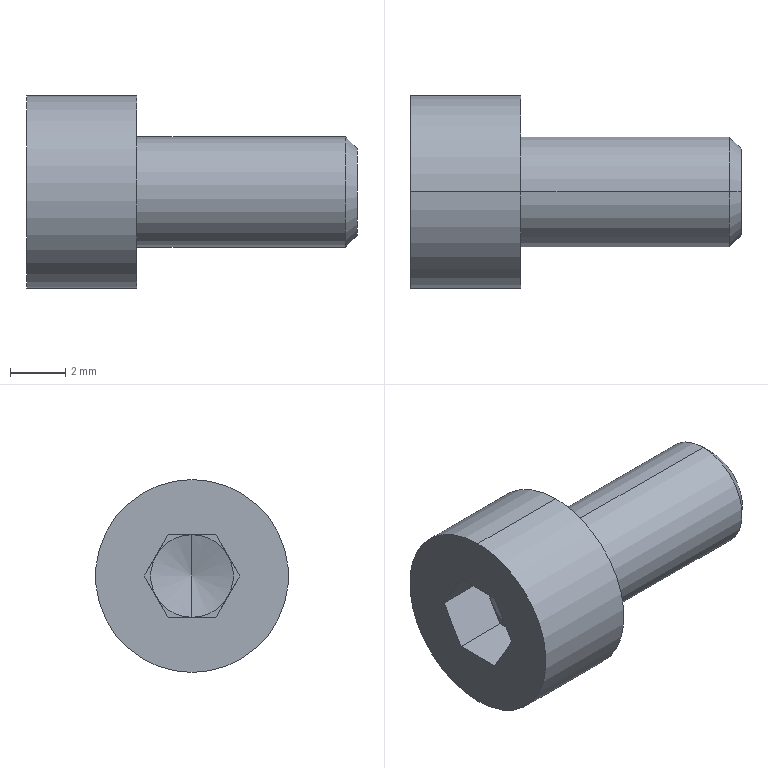Part | STEP file | 0232_303_CBM4-8 | 1 solid | 23 faces | box 12 x 7 x 7 mm | volume 236.857 mm3 | plane 15 | cylinder 4 | cone 4 | commonest cylinder face diameters 4 x2 7 x2
STEP:
#1=CARTESIAN_POINT('',(0.,0.,0.));
#2=DIRECTION('',(0.,0.,1.));
#3=DIRECTION('',(1.,0.,0.));
#4=AXIS2_PLACEMENT_3D('',#1,#2,#3);
#5=CARTESIAN_POINT('',(0.,0.,-2.));
#6=VERTEX_POINT('',#5);
#7=CARTESIAN_POINT('',(0.,0.,2.));
#8=VERTEX_POINT('',#7);
#9=CARTESIAN_POINT('',(0.,0.,0.));
#10=DIRECTION('',(1.,0.,0.));
#11=DIRECTION('',(0.,0.,-1.));
#12=AXIS2_PLACEMENT_3D('',#9,#10,#11);
#13=CIRCLE('',#12,2.);
#14=CARTESIAN_POINT('',(3.785,0.,0.));
#15=DIRECTION('',(1.,0.,0.));
#16=DIRECTION('',(0.,0.,-1.));
#17=AXIS2_PLACEMENT_3D('',#14,#15,#16);
#18=CYLINDRICAL_SURFACE('',#17,2.);
#19=CARTESIAN_POINT('',(0.,-3.785));
#20=DIRECTION('',(1.,0.));
#21=VECTOR('',#20,1.);
#22=LINE('',#19,#21);
#23=(GEOMETRIC_REPRESENTATION_CONTEXT(2)PARAMETRIC_REPRESENTATION_CONTEXT()REPRESENTATION_CONTEXT('',''));
#24=DEFINITIONAL_REPRESENTATION('',(#22),#23);
#25=PCURVE('',#18,#24);
#26=CARTESIAN_POINT('',(0.,2.75,0.));
#27=DIRECTION('',(1.,0.,0.));
#28=DIRECTION('',(0.,0.,-1.));
#29=AXIS2_PLACEMENT_3D('',#26,#27,#28);
#30=PLANE('',#29);
#31=CARTESIAN_POINT('',(0.,-2.75));
#32=DIRECTION('',(1.,0.));
#33=AXIS2_PLACEMENT_2D('',#31,#32);
#34=CIRCLE('',#33,2.);
#35=(GEOMETRIC_REPRESENTATION_CONTEXT(2)PARAMETRIC_REPRESENTATION_CONTEXT()REPRESENTATION_CONTEXT('',''));
#36=DEFINITIONAL_REPRESENTATION('',(#34),#35);
#37=PCURVE('',#30,#36);
#38=SURFACE_CURVE('',#13,(#25,#37),.PCURVE_S1.);
#39=EDGE_CURVE('',#6,#8,#38,.T.);
#40=ORIENTED_EDGE('',*,*,#39,.T.);
#41=CARTESIAN_POINT('',(7.571,0.,2.));
#42=VERTEX_POINT('',#41);
#43=CARTESIAN_POINT('',(3.785,0.,2.));
#44=DIRECTION('',(1.,0.,0.));
#45=VECTOR('',#44,1.);
#46=LINE('',#43,#45);
#47=CARTESIAN_POINT('',(3.142,0.));
#48=DIRECTION('',(0.,1.));
#49=VECTOR('',#48,1.);
#50=LINE('',#47,#49);
#51=(GEOMETRIC_REPRESENTATION_CONTEXT(2)PARAMETRIC_REPRESENTATION_CONTEXT()REPRESENTATION_CONTEXT('',''));
#52=DEFINITIONAL_REPRESENTATION('',(#50),#51);
#53=PCURVE('',#18,#52);
#54=CARTESIAN_POINT('',(3.785,0.,0.));
#55=DIRECTION('',(1.,0.,0.));
#56=DIRECTION('',(0.,0.,-1.));
#57=AXIS2_PLACEMENT_3D('',#54,#55,#56);
#58=CYLINDRICAL_SURFACE('',#57,2.);
#59=CARTESIAN_POINT('',(3.142,0.));
#60=DIRECTION('',(0.,1.));
#61=VECTOR('',#60,1.);
#62=LINE('',#59,#61);
#63=(GEOMETRIC_REPRESENTATION_CONTEXT(2)PARAMETRIC_REPRESENTATION_CONTEXT()REPRESENTATION_CONTEXT('',''));
#64=DEFINITIONAL_REPRESENTATION('',(#62),#63);
#65=PCURVE('',#58,#64);
#66=SURFACE_CURVE('',#46,(#53,#65),.PCURVE_S1.);
#67=EDGE_CURVE('',#8,#42,#66,.T.);
#68=ORIENTED_EDGE('',*,*,#67,.T.);
#69=CARTESIAN_POINT('',(7.571,0.,-2.));
#70=VERTEX_POINT('',#69);
#71=CARTESIAN_POINT('',(7.571,0.,0.));
#72=DIRECTION('',(-1.,0.,0.));
#73=DIRECTION('',(0.,0.,-1.));
#74=AXIS2_PLACEMENT_3D('',#71,#72,#73);
#75=CIRCLE('',#74,2.);
#76=CARTESIAN_POINT('',(6.283,3.785));
#77=DIRECTION('',(-1.,0.));
#78=VECTOR('',#77,1.);
#79=LINE('',#76,#78);
#80=(GEOMETRIC_REPRESENTATION_CONTEXT(2)PARAMETRIC_REPRESENTATION_CONTEXT()REPRESENTATION_CONTEXT('',''));
#81=DEFINITIONAL_REPRESENTATION('',(#79),#80);
#82=PCURVE('',#18,#81);
#83=CARTESIAN_POINT('',(7.571,0.,0.));
#84=DIRECTION('',(-1.,0.,0.));
#85=DIRECTION('',(0.,0.,1.));
#86=AXIS2_PLACEMENT_3D('',#83,#84,#85);
#87=CONICAL_SURFACE('',#86,2.,0.7854);
#88=CARTESIAN_POINT('',(-3.142,0.));
#89=DIRECTION('',(1.,0.));
#90=VECTOR('',#89,1.);
#91=LINE('',#88,#90);
#92=(GEOMETRIC_REPRESENTATION_CONTEXT(2)PARAMETRIC_REPRESENTATION_CONTEXT()REPRESENTATION_CONTEXT('',''));
#93=DEFINITIONAL_REPRESENTATION('',(#91),#92);
#94=PCURVE('',#87,#93);
#95=SURFACE_CURVE('',#75,(#82,#94),.PCURVE_S1.);
#96=EDGE_CURVE('',#42,#70,#95,.T.);
#97=ORIENTED_EDGE('',*,*,#96,.T.);
#98=CARTESIAN_POINT('',(3.785,0.,-2.));
#99=DIRECTION('',(1.,0.,0.));
#100=VECTOR('',#99,1.);
#101=LINE('',#98,#100);
#102=CARTESIAN_POINT('',(0.,0.));
#103=DIRECTION('',(0.,1.));
#104=VECTOR('',#103,1.);
#105=LINE('',#102,#104);
#106=(GEOMETRIC_REPRESENTATION_CONTEXT(2)PARAMETRIC_REPRESENTATION_CONTEXT()REPRESENTATION_CONTEXT('',''));
#107=DEFINITIONAL_REPRESENTATION('',(#105),#106);
#108=PCURVE('',#18,#107);
#109=CARTESIAN_POINT('',(6.283,0.));
#110=DIRECTION('',(0.,1.));
#111=VECTOR('',#110,1.);
#112=LINE('',#109,#111);
#113=(GEOMETRIC_REPRESENTATION_CONTEXT(2)PARAMETRIC_REPRESENTATION_CONTEXT()REPRESENTATION_CONTEXT('',''));
#114=DEFINITIONAL_REPRESENTATION('',(#112),#113);
#115=PCURVE('',#58,#114);
#116=SURFACE_CURVE('',#101,(#108,#115),.PCURVE_S1.);
#117=EDGE_CURVE('',#6,#70,#116,.T.);
#118=ORIENTED_EDGE('',*,*,#117,.F.);
#119=EDGE_LOOP('',(#40,#68,#97,#118));
#120=FACE_BOUND('',#119,.T.);
#121=ADVANCED_FACE('',(#120),#18,.T.);
#122=CARTESIAN_POINT('',(8.,0.,1.571));
#123=VERTEX_POINT('',#122);
#124=CARTESIAN_POINT('',(8.,0.,-1.571));
#125=VERTEX_POINT('',#124);
#126=CARTESIAN_POINT('',(8.,0.,0.));
#127=DIRECTION('',(-1.,0.,0.));
#128=DIRECTION('',(0.,0.,1.));
#129=AXIS2_PLACEMENT_3D('',#126,#127,#128);
#130=CIRCLE('',#129,1.571);
#131=CARTESIAN_POINT('',(0.,-0.4295));
#132=DIRECTION('',(1.,0.));
#133=VECTOR('',#132,1.);
#134=LINE('',#131,#133);
#135=(GEOMETRIC_REPRESENTATION_CONTEXT(2)PARAMETRIC_REPRESENTATION_CONTEXT()REPRESENTATION_CONTEXT('',''));
#136=DEFINITIONAL_REPRESENTATION('',(#134),#135);
#137=PCURVE('',#87,#136);
#138=CARTESIAN_POINT('',(8.,0.7853,0.));
#139=DIRECTION('',(1.,0.,0.));
#140=DIRECTION('',(0.,0.,-1.));
#141=AXIS2_PLACEMENT_3D('',#138,#139,#140);
#142=PLANE('',#141);
#143=CARTESIAN_POINT('',(-1.571,-0.7853));
#144=CARTESIAN_POINT('',(-1.571,1.935));
#145=CARTESIAN_POINT('',(0.7853,0.5748));
#146=CARTESIAN_POINT('',(3.141,-0.7853));
#147=CARTESIAN_POINT('',(0.7853,-2.145));
#148=CARTESIAN_POINT('',(-1.571,-3.505));
#149=CARTESIAN_POINT('',(-1.571,-0.7853));
#150=(BOUNDED_CURVE()B_SPLINE_CURVE(2,(#143,#144,#145,#146,#147,#148,#149),.UNSPECIFIED.,.T.,.F.)B_SPLINE_CURVE_WITH_KNOTS((1,2,2,2,2,1),(-2.094,0.,2.094,4.189,6.283,8.378),.UNSPECIFIED.)CURVE()GEOMETRIC_REPRESENTATION_ITEM()RATIONAL_B_SPLINE_CURVE((1.,0.5,1.,0.5,1.,0.5,1.))REPRESENTATION_ITEM(''));
#151=(GEOMETRIC_REPRESENTATION_CONTEXT(2)PARAMETRIC_REPRESENTATION_CONTEXT()REPRESENTATION_CONTEXT('',''));
#152=DEFINITIONAL_REPRESENTATION('',(#150),#151);
#153=PCURVE('',#142,#152);
#154=SURFACE_CURVE('',#130,(#137,#153),.PCURVE_S1.);
#155=EDGE_CURVE('',#123,#125,#154,.T.);
#156=ORIENTED_EDGE('',*,*,#155,.T.);
#157=CARTESIAN_POINT('',(7.571,0.,-2.));
#158=DIRECTION('',(-0.7071,0.,-0.7071));
#159=VECTOR('',#158,1.);
#160=LINE('',#157,#159);
#161=CARTESIAN_POINT('',(3.142,0.));
#162=DIRECTION('',(0.,1.));
#163=VECTOR('',#162,1.);
#164=LINE('',#161,#163);
#165=(GEOMETRIC_REPRESENTATION_CONTEXT(2)PARAMETRIC_REPRESENTATION_CONTEXT()REPRESENTATION_CONTEXT('',''));
#166=DEFINITIONAL_REPRESENTATION('',(#164),#165);
#167=PCURVE('',#87,#166);
#168=CARTESIAN_POINT('',(7.571,0.,0.));
#169=DIRECTION('',(-1.,0.,0.));
#170=DIRECTION('',(0.,0.,1.));
#171=AXIS2_PLACEMENT_3D('',#168,#169,#170);
#172=CONICAL_SURFACE('',#171,2.,0.7854);
#173=CARTESIAN_POINT('',(3.142,0.));
#174=DIRECTION('',(0.,1.));
#175=VECTOR('',#174,1.);
#176=LINE('',#173,#175);
#177=(GEOMETRIC_REPRESENTATION_CONTEXT(2)PARAMETRIC_REPRESENTATION_CONTEXT()REPRESENTATION_CONTEXT('',''));
#178=DEFINITIONAL_REPRESENTATION('',(#176),#177);
#179=PCURVE('',#172,#178);
#180=SURFACE_CURVE('',#160,(#167,#179),.PCURVE_S1.);
#181=EDGE_CURVE('',#125,#70,#180,.T.);
#182=ORIENTED_EDGE('',*,*,#181,.T.);
#183=ORIENTED_EDGE('',*,*,#96,.F.);
#184=CARTESIAN_POINT('',(7.571,0.,2.));
#185=DIRECTION('',(-0.7071,0.,0.7071));
#186=VECTOR('',#185,1.);
#187=LINE('',#184,#186);
#188=CARTESIAN_POINT('',(0.,0.));
#189=DIRECTION('',(0.,1.));
#190=VECTOR('',#189,1.);
#191=LINE('',#188,#190);
#192=(GEOMETRIC_REPRESENTATION_CONTEXT(2)PARAMETRIC_REPRESENTATION_CONTEXT()REPRESENTATION_CONTEXT('',''));
#193=DEFINITIONAL_REPRESENTATION('',(#191),#192);
#194=PCURVE('',#87,#193);
#195=CARTESIAN_POINT('',(6.283,0.));
#196=DIRECTION('',(0.,1.));
#197=VECTOR('',#196,1.);
#198=LINE('',#195,#197);
#199=(GEOMETRIC_REPRESENTATION_CONTEXT(2)PARAMETRIC_REPRESENTATION_CONTEXT()REPRESENTATION_CONTEXT('',''));
#200=DEFINITIONAL_REPRESENTATION('',(#198),#199);
#201=PCURVE('',#172,#200);
#202=SURFACE_CURVE('',#187,(#194,#201),.PCURVE_S1.);
#203=EDGE_CURVE('',#123,#42,#202,.T.);
#204=ORIENTED_EDGE('',*,*,#203,.F.);
#205=EDGE_LOOP('',(#156,#182,#183,#204));
#206=FACE_BOUND('',#205,.T.);
#207=ADVANCED_FACE('',(#206),#87,.T.);
#208=CARTESIAN_POINT('',(-4.,0.,-3.5));
#209=VERTEX_POINT('',#208);
#210=CARTESIAN_POINT('',(-4.,0.,3.5));
#211=VERTEX_POINT('',#210);
#212=CARTESIAN_POINT('',(-4.,0.,0.));
#213=DIRECTION('',(1.,0.,0.));
#214=DIRECTION('',(0.,0.,-1.));
#215=AXIS2_PLACEMENT_3D('',#212,#213,#214);
#216=CIRCLE('',#215,3.5);
#217=CARTESIAN_POINT('',(-2.,0.,0.));
#218=DIRECTION('',(1.,0.,0.));
#219=DIRECTION('',(0.,0.,-1.));
#220=AXIS2_PLACEMENT_3D('',#217,#218,#219);
#221=CYLINDRICAL_SURFACE('',#220,3.5);
#222=CARTESIAN_POINT('',(0.,-2.));
#223=DIRECTION('',(1.,0.));
#224=VECTOR('',#223,1.);
#225=LINE('',#222,#224);
#226=(GEOMETRIC_REPRESENTATION_CONTEXT(2)PARAMETRIC_REPRESENTATION_CONTEXT()REPRESENTATION_CONTEXT('',''));
#227=DEFINITIONAL_REPRESENTATION('',(#225),#226);
#228=PCURVE('',#221,#227);
#229=CARTESIAN_POINT('',(-4.,1.75,0.));
#230=DIRECTION('',(-1.,0.,0.));
#231=DIRECTION('',(0.,0.,1.));
#232=AXIS2_PLACEMENT_3D('',#229,#230,#231);
#233=PLANE('',#232);
#234=CARTESIAN_POINT('',(-3.5,-1.75));
#235=CARTESIAN_POINT('',(-3.5,4.312));
#236=CARTESIAN_POINT('',(1.75,1.281));
#237=CARTESIAN_POINT('',(7.,-1.75));
#238=CARTESIAN_POINT('',(1.75,-4.781));
#239=CARTESIAN_POINT('',(-3.5,-7.812));
#240=CARTESIAN_POINT('',(-3.5,-1.75));
#241=(BOUNDED_CURVE()B_SPLINE_CURVE(2,(#234,#235,#236,#237,#238,#239,#240),.UNSPECIFIED.,.T.,.F.)B_SPLINE_CURVE_WITH_KNOTS((1,2,2,2,2,1),(-2.094,0.,2.094,4.189,6.283,8.378),.UNSPECIFIED.)CURVE()GEOMETRIC_REPRESENTATION_ITEM()RATIONAL_B_SPLINE_CURVE((1.,0.5,1.,0.5,1.,0.5,1.))REPRESENTATION_ITEM(''));
#242=(GEOMETRIC_REPRESENTATION_CONTEXT(2)PARAMETRIC_REPRESENTATION_CONTEXT()REPRESENTATION_CONTEXT('',''));
#243=DEFINITIONAL_REPRESENTATION('',(#241),#242);
#244=PCURVE('',#233,#243);
#245=SURFACE_CURVE('',#216,(#228,#244),.PCURVE_S1.);
#246=EDGE_CURVE('',#209,#211,#245,.T.);
#247=ORIENTED_EDGE('',*,*,#246,.T.);
#248=CARTESIAN_POINT('',(0.,0.,3.5));
#249=VERTEX_POINT('',#248);
#250=CARTESIAN_POINT('',(-2.,0.,3.5));
#251=DIRECTION('',(1.,0.,0.));
#252=VECTOR('',#251,1.);
#253=LINE('',#250,#252);
#254=CARTESIAN_POINT('',(3.142,0.));
#255=DIRECTION('',(0.,1.));
#256=VECTOR('',#255,1.);
#257=LINE('',#254,#256);
#258=(GEOMETRIC_REPRESENTATION_CONTEXT(2)PARAMETRIC_REPRESENTATION_CONTEXT()REPRESENTATION_CONTEXT('',''));
#259=DEFINITIONAL_REPRESENTATION('',(#257),#258);
#260=PCURVE('',#221,#259);
#261=CARTESIAN_POINT('',(-2.,0.,0.));
#262=DIRECTION('',(1.,0.,0.));
#263=DIRECTION('',(0.,0.,-1.));
#264=AXIS2_PLACEMENT_3D('',#261,#262,#263);
#265=CYLINDRICAL_SURFACE('',#264,3.5);
#266=CARTESIAN_POINT('',(3.142,0.));
#267=DIRECTION('',(0.,1.));
#268=VECTOR('',#267,1.);
#269=LINE('',#266,#268);
#270=(GEOMETRIC_REPRESENTATION_CONTEXT(2)PARAMETRIC_REPRESENTATION_CONTEXT()REPRESENTATION_CONTEXT('',''));
#271=DEFINITIONAL_REPRESENTATION('',(#269),#270);
#272=PCURVE('',#265,#271);
#273=SURFACE_CURVE('',#253,(#260,#272),.PCURVE_S1.);
#274=EDGE_CURVE('',#211,#249,#273,.T.);
#275=ORIENTED_EDGE('',*,*,#274,.T.);
#276=CARTESIAN_POINT('',(0.,0.,-3.5));
#277=VERTEX_POINT('',#276);
#278=CARTESIAN_POINT('',(0.,0.,0.));
#279=DIRECTION('',(1.,0.,0.));
#280=DIRECTION('',(0.,0.,-1.));
#281=AXIS2_PLACEMENT_3D('',#278,#279,#280);
#282=CIRCLE('',#281,3.5);
#283=CARTESIAN_POINT('',(0.,2.));
#284=DIRECTION('',(1.,0.));
#285=VECTOR('',#284,1.);
#286=LINE('',#283,#285);
#287=(GEOMETRIC_REPRESENTATION_CONTEXT(2)PARAMETRIC_REPRESENTATION_CONTEXT()REPRESENTATION_CONTEXT('',''));
#288=DEFINITIONAL_REPRESENTATION('',(#286),#287);
#289=PCURVE('',#221,#288);
#290=CARTESIAN_POINT('',(0.,-2.75));
#291=DIRECTION('',(1.,0.));
#292=AXIS2_PLACEMENT_2D('',#290,#291);
#293=CIRCLE('',#292,3.5);
#294=(GEOMETRIC_REPRESENTATION_CONTEXT(2)PARAMETRIC_REPRESENTATION_CONTEXT()REPRESENTATION_CONTEXT('',''));
#295=DEFINITIONAL_REPRESENTATION('',(#293),#294);
#296=PCURVE('',#30,#295);
#297=SURFACE_CURVE('',#282,(#289,#296),.PCURVE_S1.);
#298=EDGE_CURVE('',#277,#249,#297,.T.);
#299=ORIENTED_EDGE('',*,*,#298,.F.);
#300=CARTESIAN_POINT('',(-2.,0.,-3.5));
#301=DIRECTION('',(1.,0.,0.));
#302=VECTOR('',#301,1.);
#303=LINE('',#300,#302);
#304=CARTESIAN_POINT('',(0.,0.));
#305=DIRECTION('',(0.,1.));
#306=VECTOR('',#305,1.);
#307=LINE('',#304,#306);
#308=(GEOMETRIC_REPRESENTATION_CONTEXT(2)PARAMETRIC_REPRESENTATION_CONTEXT()REPRESENTATION_CONTEXT('',''));
#309=DEFINITIONAL_REPRESENTATION('',(#307),#308);
#310=PCURVE('',#221,#309);
#311=CARTESIAN_POINT('',(6.283,0.));
#312=DIRECTION('',(0.,1.));
#313=VECTOR('',#312,1.);
#314=LINE('',#311,#313);
#315=(GEOMETRIC_REPRESENTATION_CONTEXT(2)PARAMETRIC_REPRESENTATION_CONTEXT()REPRESENTATION_CONTEXT('',''));
#316=DEFINITIONAL_REPRESENTATION('',(#314),#315);
#317=PCURVE('',#265,#316);
#318=SURFACE_CURVE('',#303,(#310,#317),.PCURVE_S1.);
#319=EDGE_CURVE('',#209,#277,#318,.T.);
#320=ORIENTED_EDGE('',*,*,#319,.F.);
#321=EDGE_LOOP('',(#247,#275,#299,#320));
#322=FACE_BOUND('',#321,.T.);
#323=ADVANCED_FACE('',(#322),#221,.T.);
#324=CARTESIAN_POINT('',(-2.,0.,1.5));
#325=VERTEX_POINT('',#324);
#326=CARTESIAN_POINT('',(-2.,-1.299,0.75));
#327=VERTEX_POINT('',#326);
#328=CARTESIAN_POINT('',(-2.,0.,0.));
#329=DIRECTION('',(1.,0.,0.));
#330=DIRECTION('',(0.,0.,1.));
#331=AXIS2_PLACEMENT_3D('',#328,#329,#330);
#332=CIRCLE('',#331,1.5);
#333=CARTESIAN_POINT('',(-2.,0.,0.));
#334=DIRECTION('',(-1.,0.,0.));
#335=DIRECTION('',(0.,0.,1.));
#336=AXIS2_PLACEMENT_3D('',#333,#334,#335);
#337=CONICAL_SURFACE('',#336,1.5,1.309);
#338=CARTESIAN_POINT('',(6.283,0.));
#339=DIRECTION('',(-1.,0.));
#340=VECTOR('',#339,1.);
#341=LINE('',#338,#340);
#342=(GEOMETRIC_REPRESENTATION_CONTEXT(2)PARAMETRIC_REPRESENTATION_CONTEXT()REPRESENTATION_CONTEXT('',''));
#343=DEFINITIONAL_REPRESENTATION('',(#341),#342);
#344=PCURVE('',#337,#343);
#345=CARTESIAN_POINT('',(-2.,0.,0.));
#346=DIRECTION('',(1.,0.,0.));
#347=DIRECTION('',(0.,0.,-1.));
#348=AXIS2_PLACEMENT_3D('',#345,#346,#347);
#349=PLANE('',#348);
#350=CARTESIAN_POINT('',(0.,0.));
#351=DIRECTION('',(-1.,0.));
#352=AXIS2_PLACEMENT_2D('',#350,#351);
#353=CIRCLE('',#352,1.5);
#354=(GEOMETRIC_REPRESENTATION_CONTEXT(2)PARAMETRIC_REPRESENTATION_CONTEXT()REPRESENTATION_CONTEXT('',''));
#355=DEFINITIONAL_REPRESENTATION('',(#353),#354);
#356=PCURVE('',#349,#355);
#357=SURFACE_CURVE('',#332,(#344,#356),.PCURVE_S1.);
#358=EDGE_CURVE('',#325,#327,#357,.T.);
#359=ORIENTED_EDGE('',*,*,#358,.T.);
#360=CARTESIAN_POINT('',(-2.,-1.299,-0.75));
#361=VERTEX_POINT('',#360);
#362=CARTESIAN_POINT('',(-2.,0.,0.));
#363=DIRECTION('',(1.,0.,0.));
#364=DIRECTION('',(0.,0.,1.));
#365=AXIS2_PLACEMENT_3D('',#362,#363,#364);
#366=CIRCLE('',#365,1.5);
#367=CARTESIAN_POINT('',(6.283,0.));
#368=DIRECTION('',(-1.,0.));
#369=VECTOR('',#368,1.);
#370=LINE('',#367,#369);
#371=(GEOMETRIC_REPRESENTATION_CONTEXT(2)PARAMETRIC_REPRESENTATION_CONTEXT()REPRESENTATION_CONTEXT('',''));
#372=DEFINITIONAL_REPRESENTATION('',(#370),#371);
#373=PCURVE('',#337,#372);
#374=CARTESIAN_POINT('',(-2.,0.,0.));
#375=DIRECTION('',(1.,0.,0.));
#376=DIRECTION('',(0.,0.,-1.));
#377=AXIS2_PLACEMENT_3D('',#374,#375,#376);
#378=PLANE('',#377);
#379=CARTESIAN_POINT('',(0.,0.));
#380=DIRECTION('',(-1.,0.));
#381=AXIS2_PLACEMENT_2D('',#379,#380);
#382=CIRCLE('',#381,1.5);
#383=(GEOMETRIC_REPRESENTATION_CONTEXT(2)PARAMETRIC_REPRESENTATION_CONTEXT()REPRESENTATION_CONTEXT('',''));
#384=DEFINITIONAL_REPRESENTATION('',(#382),#383);
#385=PCURVE('',#378,#384);
#386=SURFACE_CURVE('',#366,(#373,#385),.PCURVE_S1.);
#387=EDGE_CURVE('',#327,#361,#386,.T.);
#388=ORIENTED_EDGE('',*,*,#387,.T.);
#389=CARTESIAN_POINT('',(-2.,0.,-1.5));
#390=VERTEX_POINT('',#389);
#391=CARTESIAN_POINT('',(-2.,0.,0.));
#392=DIRECTION('',(-1.,0.,0.));
#393=DIRECTION('',(0.,0.,1.));
#394=AXIS2_PLACEMENT_3D('',#391,#392,#393);
#395=CIRCLE('',#394,1.5);
#396=CARTESIAN_POINT('',(0.,0.));
#397=DIRECTION('',(1.,0.));
#398=VECTOR('',#397,1.);
#399=LINE('',#396,#398);
#400=(GEOMETRIC_REPRESENTATION_CONTEXT(2)PARAMETRIC_REPRESENTATION_CONTEXT()REPRESENTATION_CONTEXT('',''));
#401=DEFINITIONAL_REPRESENTATION('',(#399),#400);
#402=PCURVE('',#337,#401);
#403=CARTESIAN_POINT('',(-2.,0.,0.));
#404=DIRECTION('',(1.,0.,0.));
#405=DIRECTION('',(0.,0.,-1.));
#406=AXIS2_PLACEMENT_3D('',#403,#404,#405);
#407=PLANE('',#406);
#408=CARTESIAN_POINT('',(-1.5,0.));
#409=CARTESIAN_POINT('',(-1.5,2.598));
#410=CARTESIAN_POINT('',(0.75,1.299));
#411=CARTESIAN_POINT('',(3.,0.));
#412=CARTESIAN_POINT('',(0.75,-1.299));
#413=CARTESIAN_POINT('',(-1.5,-2.598));
#414=CARTESIAN_POINT('',(-1.5,0.));
#415=(BOUNDED_CURVE()B_SPLINE_CURVE(2,(#408,#409,#410,#411,#412,#413,#414),.UNSPECIFIED.,.T.,.F.)B_SPLINE_CURVE_WITH_KNOTS((1,2,2,2,2,1),(-2.094,0.,2.094,4.189,6.283,8.378),.UNSPECIFIED.)CURVE()GEOMETRIC_REPRESENTATION_ITEM()RATIONAL_B_SPLINE_CURVE((1.,0.5,1.,0.5,1.,0.5,1.))REPRESENTATION_ITEM(''));
#416=(GEOMETRIC_REPRESENTATION_CONTEXT(2)PARAMETRIC_REPRESENTATION_CONTEXT()REPRESENTATION_CONTEXT('',''));
#417=DEFINITIONAL_REPRESENTATION('',(#415),#416);
#418=PCURVE('',#407,#417);
#419=SURFACE_CURVE('',#395,(#402,#418),.PCURVE_S1.);
#420=EDGE_CURVE('',#390,#361,#419,.T.);
#421=ORIENTED_EDGE('',*,*,#420,.F.);
#422=CARTESIAN_POINT('',(-1.598,0.000000001,0.));
#423=VERTEX_POINT('',#422);
#424=CARTESIAN_POINT('',(-2.,0.,-1.5));
#425=DIRECTION('',(-0.2588,0.,-0.9659));
#426=VECTOR('',#425,1.);
#427=LINE('',#424,#426);
#428=CARTESIAN_POINT('',(3.142,0.));
#429=DIRECTION('',(0.,1.));
#430=VECTOR('',#429,1.);
#431=LINE('',#428,#430);
#432=(GEOMETRIC_REPRESENTATION_CONTEXT(2)PARAMETRIC_REPRESENTATION_CONTEXT()REPRESENTATION_CONTEXT('',''));
#433=DEFINITIONAL_REPRESENTATION('',(#431),#432);
#434=PCURVE('',#337,#433);
#435=CARTESIAN_POINT('',(-2.,0.,0.));
#436=DIRECTION('',(-1.,0.,0.));
#437=DIRECTION('',(0.,0.,1.));
#438=AXIS2_PLACEMENT_3D('',#435,#436,#437);
#439=CONICAL_SURFACE('',#438,1.5,1.309);
#440=CARTESIAN_POINT('',(3.142,0.));
#441=DIRECTION('',(0.,1.));
#442=VECTOR('',#441,1.);
#443=LINE('',#440,#442);
#444=(GEOMETRIC_REPRESENTATION_CONTEXT(2)PARAMETRIC_REPRESENTATION_CONTEXT()REPRESENTATION_CONTEXT('',''));
#445=DEFINITIONAL_REPRESENTATION('',(#443),#444);
#446=PCURVE('',#439,#445);
#447=SURFACE_CURVE('',#427,(#434,#446),.PCURVE_S1.);
#448=EDGE_CURVE('',#423,#390,#447,.T.);
#449=ORIENTED_EDGE('',*,*,#448,.F.);
#450=CARTESIAN_POINT('',(-2.,0.,1.5));
#451=DIRECTION('',(-0.2588,0.,0.9659));
#452=VECTOR('',#451,1.);
#453=LINE('',#450,#452);
#454=CARTESIAN_POINT('',(6.283,0.));
#455=DIRECTION('',(0.,1.));
#456=VECTOR('',#455,1.);
#457=LINE('',#454,#456);
#458=(GEOMETRIC_REPRESENTATION_CONTEXT(2)PARAMETRIC_REPRESENTATION_CONTEXT()REPRESENTATION_CONTEXT('',''));
#459=DEFINITIONAL_REPRESENTATION('',(#457),#458);
#460=PCURVE('',#337,#459);
#461=CARTESIAN_POINT('',(0.,0.));
#462=DIRECTION('',(0.,1.));
#463=VECTOR('',#462,1.);
#464=LINE('',#461,#463);
#465=(GEOMETRIC_REPRESENTATION_CONTEXT(2)PARAMETRIC_REPRESENTATION_CONTEXT()REPRESENTATION_CONTEXT('',''));
#466=DEFINITIONAL_REPRESENTATION('',(#464),#465);
#467=PCURVE('',#439,#466);
#468=SURFACE_CURVE('',#453,(#460,#467),.PCURVE_S1.);
#469=EDGE_CURVE('',#423,#325,#468,.T.);
#470=ORIENTED_EDGE('',*,*,#469,.T.);
#471=EDGE_LOOP('',(#359,#388,#421,#449,#470));
#472=FACE_BOUND('',#471,.F.);
#473=ADVANCED_FACE('',(#472),#337,.F.);
#474=ORIENTED_EDGE('',*,*,#67,.F.);
#475=CARTESIAN_POINT('',(0.,0.,0.));
#476=DIRECTION('',(1.,0.,0.));
#477=DIRECTION('',(0.,0.,-1.));
#478=AXIS2_PLACEMENT_3D('',#475,#476,#477);
#479=CIRCLE('',#478,2.);
#480=CARTESIAN_POINT('',(0.,-3.785));
#481=DIRECTION('',(1.,0.));
#482=VECTOR('',#481,1.);
#483=LINE('',#480,#482);
#484=(GEOMETRIC_REPRESENTATION_CONTEXT(2)PARAMETRIC_REPRESENTATION_CONTEXT()REPRESENTATION_CONTEXT('',''));
#485=DEFINITIONAL_REPRESENTATION('',(#483),#484);
#486=PCURVE('',#58,#485);
#487=CARTESIAN_POINT('',(0.,-2.75));
#488=DIRECTION('',(1.,0.));
#489=AXIS2_PLACEMENT_2D('',#487,#488);
#490=CIRCLE('',#489,2.);
#491=(GEOMETRIC_REPRESENTATION_CONTEXT(2)PARAMETRIC_REPRESENTATION_CONTEXT()REPRESENTATION_CONTEXT('',''));
#492=DEFINITIONAL_REPRESENTATION('',(#490),#491);
#493=PCURVE('',#30,#492);
#494=SURFACE_CURVE('',#479,(#486,#493),.PCURVE_S1.);
#495=EDGE_CURVE('',#8,#6,#494,.T.);
#496=ORIENTED_EDGE('',*,*,#495,.T.);
#497=ORIENTED_EDGE('',*,*,#117,.T.);
#498=CARTESIAN_POINT('',(7.571,0.,0.));
#499=DIRECTION('',(-1.,0.,0.));
#500=DIRECTION('',(0.,0.,-1.));
#501=AXIS2_PLACEMENT_3D('',#498,#499,#500);
#502=CIRCLE('',#501,2.);
#503=CARTESIAN_POINT('',(6.283,3.785));
#504=DIRECTION('',(-1.,0.));
#505=VECTOR('',#504,1.);
#506=LINE('',#503,#505);
#507=(GEOMETRIC_REPRESENTATION_CONTEXT(2)PARAMETRIC_REPRESENTATION_CONTEXT()REPRESENTATION_CONTEXT('',''));
#508=DEFINITIONAL_REPRESENTATION('',(#506),#507);
#509=PCURVE('',#58,#508);
#510=CARTESIAN_POINT('',(3.142,0.));
#511=DIRECTION('',(1.,0.));
#512=VECTOR('',#511,1.);
#513=LINE('',#510,#512);
#514=(GEOMETRIC_REPRESENTATION_CONTEXT(2)PARAMETRIC_REPRESENTATION_CONTEXT()REPRESENTATION_CONTEXT('',''));
#515=DEFINITIONAL_REPRESENTATION('',(#513),#514);
#516=PCURVE('',#172,#515);
#517=SURFACE_CURVE('',#502,(#509,#516),.PCURVE_S1.);
#518=EDGE_CURVE('',#70,#42,#517,.T.);
#519=ORIENTED_EDGE('',*,*,#518,.T.);
#520=EDGE_LOOP('',(#474,#496,#497,#519));
#521=FACE_BOUND('',#520,.T.);
#522=ADVANCED_FACE('',(#521),#58,.T.);
#523=ORIENTED_EDGE('',*,*,#39,.F.);
#524=ORIENTED_EDGE('',*,*,#495,.F.);
#525=EDGE_LOOP('',(#523,#524));
#526=FACE_BOUND('',#525,.T.);
#527=ORIENTED_EDGE('',*,*,#298,.T.);
#528=CARTESIAN_POINT('',(0.,0.,0.));
#529=DIRECTION('',(1.,0.,0.));
#530=DIRECTION('',(0.,0.,-1.));
#531=AXIS2_PLACEMENT_3D('',#528,#529,#530);
#532=CIRCLE('',#531,3.5);
#533=CARTESIAN_POINT('',(0.,-2.75));
#534=DIRECTION('',(1.,0.));
#535=AXIS2_PLACEMENT_2D('',#533,#534);
#536=CIRCLE('',#535,3.5);
#537=(GEOMETRIC_REPRESENTATION_CONTEXT(2)PARAMETRIC_REPRESENTATION_CONTEXT()REPRESENTATION_CONTEXT('',''));
#538=DEFINITIONAL_REPRESENTATION('',(#536),#537);
#539=PCURVE('',#30,#538);
#540=CARTESIAN_POINT('',(0.,2.));
#541=DIRECTION('',(1.,0.));
#542=VECTOR('',#541,1.);
#543=LINE('',#540,#542);
#544=(GEOMETRIC_REPRESENTATION_CONTEXT(2)PARAMETRIC_REPRESENTATION_CONTEXT()REPRESENTATION_CONTEXT('',''));
#545=DEFINITIONAL_REPRESENTATION('',(#543),#544);
#546=PCURVE('',#265,#545);
#547=SURFACE_CURVE('',#532,(#539,#546),.PCURVE_S1.);
#548=EDGE_CURVE('',#249,#277,#547,.T.);
#549=ORIENTED_EDGE('',*,*,#548,.T.);
#550=EDGE_LOOP('',(#527,#549));
#551=FACE_BOUND('',#550,.T.);
#552=ADVANCED_FACE('',(#526,#551),#30,.T.);
#553=ORIENTED_EDGE('',*,*,#181,.F.);
#554=CARTESIAN_POINT('',(8.,0.,0.));
#555=DIRECTION('',(-1.,0.,0.));
#556=DIRECTION('',(0.,0.,1.));
#557=AXIS2_PLACEMENT_3D('',#554,#555,#556);
#558=CIRCLE('',#557,1.571);
#559=CARTESIAN_POINT('',(0.,-0.4295));
#560=DIRECTION('',(1.,0.));
#561=VECTOR('',#560,1.);
#562=LINE('',#559,#561);
#563=(GEOMETRIC_REPRESENTATION_CONTEXT(2)PARAMETRIC_REPRESENTATION_CONTEXT()REPRESENTATION_CONTEXT('',''));
#564=DEFINITIONAL_REPRESENTATION('',(#562),#563);
#565=PCURVE('',#172,#564);
#566=CARTESIAN_POINT('',(-1.571,-0.7853));
#567=CARTESIAN_POINT('',(-1.571,1.935));
#568=CARTESIAN_POINT('',(0.7853,0.5748));
#569=CARTESIAN_POINT('',(3.141,-0.7853));
#570=CARTESIAN_POINT('',(0.7853,-2.145));
#571=CARTESIAN_POINT('',(-1.571,-3.505));
#572=CARTESIAN_POINT('',(-1.571,-0.7853));
#573=(BOUNDED_CURVE()B_SPLINE_CURVE(2,(#566,#567,#568,#569,#570,#571,#572),.UNSPECIFIED.,.T.,.F.)B_SPLINE_CURVE_WITH_KNOTS((1,2,2,2,2,1),(-2.094,0.,2.094,4.189,6.283,8.378),.UNSPECIFIED.)CURVE()GEOMETRIC_REPRESENTATION_ITEM()RATIONAL_B_SPLINE_CURVE((1.,0.5,1.,0.5,1.,0.5,1.))REPRESENTATION_ITEM(''));
#574=(GEOMETRIC_REPRESENTATION_CONTEXT(2)PARAMETRIC_REPRESENTATION_CONTEXT()REPRESENTATION_CONTEXT('',''));
#575=DEFINITIONAL_REPRESENTATION('',(#573),#574);
#576=PCURVE('',#142,#575);
#577=SURFACE_CURVE('',#558,(#565,#576),.PCURVE_S1.);
#578=EDGE_CURVE('',#125,#123,#577,.T.);
#579=ORIENTED_EDGE('',*,*,#578,.T.);
#580=ORIENTED_EDGE('',*,*,#203,.T.);
#581=ORIENTED_EDGE('',*,*,#518,.F.);
#582=EDGE_LOOP('',(#553,#579,#580,#581));
#583=FACE_BOUND('',#582,.T.);
#584=ADVANCED_FACE('',(#583),#172,.T.);
#585=ORIENTED_EDGE('',*,*,#274,.F.);
#586=CARTESIAN_POINT('',(-4.,0.,0.));
#587=DIRECTION('',(1.,0.,0.));
#588=DIRECTION('',(0.,0.,-1.));
#589=AXIS2_PLACEMENT_3D('',#586,#587,#588);
#590=CIRCLE('',#589,3.5);
#591=CARTESIAN_POINT('',(0.,-2.));
#592=DIRECTION('',(1.,0.));
#593=VECTOR('',#592,1.);
#594=LINE('',#591,#593);
#595=(GEOMETRIC_REPRESENTATION_CONTEXT(2)PARAMETRIC_REPRESENTATION_CONTEXT()REPRESENTATION_CONTEXT('',''));
#596=DEFINITIONAL_REPRESENTATION('',(#594),#595);
#597=PCURVE('',#265,#596);
#598=CARTESIAN_POINT('',(-3.5,-1.75));
#599=CARTESIAN_POINT('',(-3.5,4.312));
#600=CARTESIAN_POINT('',(1.75,1.281));
#601=CARTESIAN_POINT('',(7.,-1.75));
#602=CARTESIAN_POINT('',(1.75,-4.781));
#603=CARTESIAN_POINT('',(-3.5,-7.812));
#604=CARTESIAN_POINT('',(-3.5,-1.75));
#605=(BOUNDED_CURVE()B_SPLINE_CURVE(2,(#598,#599,#600,#601,#602,#603,#604),.UNSPECIFIED.,.T.,.F.)B_SPLINE_CURVE_WITH_KNOTS((1,2,2,2,2,1),(-2.094,0.,2.094,4.189,6.283,8.378),.UNSPECIFIED.)CURVE()GEOMETRIC_REPRESENTATION_ITEM()RATIONAL_B_SPLINE_CURVE((1.,0.5,1.,0.5,1.,0.5,1.))REPRESENTATION_ITEM(''));
#606=(GEOMETRIC_REPRESENTATION_CONTEXT(2)PARAMETRIC_REPRESENTATION_CONTEXT()REPRESENTATION_CONTEXT('',''));
#607=DEFINITIONAL_REPRESENTATION('',(#605),#606);
#608=PCURVE('',#233,#607);
#609=SURFACE_CURVE('',#590,(#597,#608),.PCURVE_S1.);
#610=EDGE_CURVE('',#211,#209,#609,.T.);
#611=ORIENTED_EDGE('',*,*,#610,.T.);
#612=ORIENTED_EDGE('',*,*,#319,.T.);
#613=ORIENTED_EDGE('',*,*,#548,.F.);
#614=EDGE_LOOP('',(#585,#611,#612,#613));
#615=FACE_BOUND('',#614,.T.);
#616=ADVANCED_FACE('',(#615),#265,.T.);
#617=ORIENTED_EDGE('',*,*,#155,.F.);
#618=ORIENTED_EDGE('',*,*,#578,.F.);
#619=EDGE_LOOP('',(#617,#618));
#620=FACE_BOUND('',#619,.T.);
#621=ADVANCED_FACE('',(#620),#142,.T.);
#622=ORIENTED_EDGE('',*,*,#246,.F.);
#623=ORIENTED_EDGE('',*,*,#610,.F.);
#624=EDGE_LOOP('',(#622,#623));
#625=FACE_BOUND('',#624,.T.);
#626=CARTESIAN_POINT('',(-4.,0.866,-1.5));
#627=VERTEX_POINT('',#626);
#628=CARTESIAN_POINT('',(-4.,1.732,0.));
#629=VERTEX_POINT('',#628);
#630=CARTESIAN_POINT('',(-4.,1.732,0.));
#631=DIRECTION('',(0.,0.5,0.866));
#632=VECTOR('',#631,1.);
#633=LINE('',#630,#632);
#634=CARTESIAN_POINT('',(0.,-0.01795));
#635=DIRECTION('',(0.866,0.5));
#636=VECTOR('',#635,1.);
#637=LINE('',#634,#636);
#638=(GEOMETRIC_REPRESENTATION_CONTEXT(2)PARAMETRIC_REPRESENTATION_CONTEXT()REPRESENTATION_CONTEXT('',''));
#639=DEFINITIONAL_REPRESENTATION('',(#637),#638);
#640=PCURVE('',#233,#639);
#641=CARTESIAN_POINT('',(-4.,1.732,0.));
#642=DIRECTION('',(0.,0.866,-0.5));
#643=DIRECTION('',(0.,0.5,0.866));
#644=AXIS2_PLACEMENT_3D('',#641,#642,#643);
#645=PLANE('',#644);
#646=CARTESIAN_POINT('',(0.,0.));
#647=DIRECTION('',(1.,0.));
#648=VECTOR('',#647,1.);
#649=LINE('',#646,#648);
#650=(GEOMETRIC_REPRESENTATION_CONTEXT(2)PARAMETRIC_REPRESENTATION_CONTEXT()REPRESENTATION_CONTEXT('',''));
#651=DEFINITIONAL_REPRESENTATION('',(#649),#650);
#652=PCURVE('',#645,#651);
#653=SURFACE_CURVE('',#633,(#640,#652),.PCURVE_S1.);
#654=EDGE_CURVE('',#627,#629,#653,.T.);
#655=ORIENTED_EDGE('',*,*,#654,.T.);
#656=CARTESIAN_POINT('',(-4.,0.866,1.5));
#657=VERTEX_POINT('',#656);
#658=CARTESIAN_POINT('',(-4.,1.732,0.));
#659=DIRECTION('',(0.,-0.5,0.866));
#660=VECTOR('',#659,1.);
#661=LINE('',#658,#660);
#662=CARTESIAN_POINT('',(0.,-0.01795));
#663=DIRECTION('',(0.866,-0.5));
#664=VECTOR('',#663,1.);
#665=LINE('',#662,#664);
#666=(GEOMETRIC_REPRESENTATION_CONTEXT(2)PARAMETRIC_REPRESENTATION_CONTEXT()REPRESENTATION_CONTEXT('',''));
#667=DEFINITIONAL_REPRESENTATION('',(#665),#666);
#668=PCURVE('',#233,#667);
#669=CARTESIAN_POINT('',(-4.,0.866,1.5));
#670=DIRECTION('',(0.,0.866,0.5));
#671=DIRECTION('',(0.,-0.5,0.866));
#672=AXIS2_PLACEMENT_3D('',#669,#670,#671);
#673=PLANE('',#672);
#674=CARTESIAN_POINT('',(-1.732,0.));
#675=DIRECTION('',(1.,0.));
#676=VECTOR('',#675,1.);
#677=LINE('',#674,#676);
#678=(GEOMETRIC_REPRESENTATION_CONTEXT(2)PARAMETRIC_REPRESENTATION_CONTEXT()REPRESENTATION_CONTEXT('',''));
#679=DEFINITIONAL_REPRESENTATION('',(#677),#678);
#680=PCURVE('',#673,#679);
#681=SURFACE_CURVE('',#661,(#668,#680),.PCURVE_S1.);
#682=EDGE_CURVE('',#629,#657,#681,.T.);
#683=ORIENTED_EDGE('',*,*,#682,.T.);
#684=CARTESIAN_POINT('',(-4.,-0.866,1.5));
#685=VERTEX_POINT('',#684);
#686=CARTESIAN_POINT('',(-4.,-0.866,1.5));
#687=DIRECTION('',(0.,-1.,0.));
#688=VECTOR('',#687,1.);
#689=LINE('',#686,#688);
#690=CARTESIAN_POINT('',(1.5,-2.616));
#691=DIRECTION('',(0.,-1.));
#692=VECTOR('',#691,1.);
#693=LINE('',#690,#692);
#694=(GEOMETRIC_REPRESENTATION_CONTEXT(2)PARAMETRIC_REPRESENTATION_CONTEXT()REPRESENTATION_CONTEXT('',''));
#695=DEFINITIONAL_REPRESENTATION('',(#693),#694);
#696=PCURVE('',#233,#695);
#697=CARTESIAN_POINT('',(-4.,-0.866,1.5));
#698=DIRECTION('',(0.,0.,1.));
#699=DIRECTION('',(1.,0.,0.));
#700=AXIS2_PLACEMENT_3D('',#697,#698,#699);
#701=PLANE('',#700);
#702=CARTESIAN_POINT('',(0.,0.));
#703=DIRECTION('',(0.,-1.));
#704=VECTOR('',#703,1.);
#705=LINE('',#702,#704);
#706=(GEOMETRIC_REPRESENTATION_CONTEXT(2)PARAMETRIC_REPRESENTATION_CONTEXT()REPRESENTATION_CONTEXT('',''));
#707=DEFINITIONAL_REPRESENTATION('',(#705),#706);
#708=PCURVE('',#701,#707);
#709=SURFACE_CURVE('',#689,(#696,#708),.PCURVE_S1.);
#710=EDGE_CURVE('',#657,#685,#709,.T.);
#711=ORIENTED_EDGE('',*,*,#710,.T.);
#712=CARTESIAN_POINT('',(-4.,-1.732,0.));
#713=VERTEX_POINT('',#712);
#714=CARTESIAN_POINT('',(-4.,-1.732,0.));
#715=DIRECTION('',(0.,-0.5,-0.866));
#716=VECTOR('',#715,1.);
#717=LINE('',#714,#716);
#718=CARTESIAN_POINT('',(0.,-3.482));
#719=DIRECTION('',(-0.866,-0.5));
#720=VECTOR('',#719,1.);
#721=LINE('',#718,#720);
#722=(GEOMETRIC_REPRESENTATION_CONTEXT(2)PARAMETRIC_REPRESENTATION_CONTEXT()REPRESENTATION_CONTEXT('',''));
#723=DEFINITIONAL_REPRESENTATION('',(#721),#722);
#724=PCURVE('',#233,#723);
#725=CARTESIAN_POINT('',(-4.,-1.732,0.));
#726=DIRECTION('',(0.,-0.866,0.5));
#727=DIRECTION('',(0.,-0.5,-0.866));
#728=AXIS2_PLACEMENT_3D('',#725,#726,#727);
#729=PLANE('',#728);
#730=CARTESIAN_POINT('',(0.,0.));
#731=DIRECTION('',(1.,0.));
#732=VECTOR('',#731,1.);
#733=LINE('',#730,#732);
#734=(GEOMETRIC_REPRESENTATION_CONTEXT(2)PARAMETRIC_REPRESENTATION_CONTEXT()REPRESENTATION_CONTEXT('',''));
#735=DEFINITIONAL_REPRESENTATION('',(#733),#734);
#736=PCURVE('',#729,#735);
#737=SURFACE_CURVE('',#717,(#724,#736),.PCURVE_S1.);
#738=EDGE_CURVE('',#685,#713,#737,.T.);
#739=ORIENTED_EDGE('',*,*,#738,.T.);
#740=CARTESIAN_POINT('',(-4.,-0.866,-1.5));
#741=VERTEX_POINT('',#740);
#742=CARTESIAN_POINT('',(-4.,-0.866,-1.5));
#743=DIRECTION('',(0.,0.5,-0.866));
#744=VECTOR('',#743,1.);
#745=LINE('',#742,#744);
#746=CARTESIAN_POINT('',(-1.5,-2.616));
#747=DIRECTION('',(-0.866,0.5));
#748=VECTOR('',#747,1.);
#749=LINE('',#746,#748);
#750=(GEOMETRIC_REPRESENTATION_CONTEXT(2)PARAMETRIC_REPRESENTATION_CONTEXT()REPRESENTATION_CONTEXT('',''));
#751=DEFINITIONAL_REPRESENTATION('',(#749),#750);
#752=PCURVE('',#233,#751);
#753=CARTESIAN_POINT('',(-4.,-0.866,-1.5));
#754=DIRECTION('',(0.,-0.866,-0.5));
#755=DIRECTION('',(0.,0.5,-0.866));
#756=AXIS2_PLACEMENT_3D('',#753,#754,#755);
#757=PLANE('',#756);
#758=CARTESIAN_POINT('',(0.,0.));
#759=DIRECTION('',(1.,0.));
#760=VECTOR('',#759,1.);
#761=LINE('',#758,#760);
#762=(GEOMETRIC_REPRESENTATION_CONTEXT(2)PARAMETRIC_REPRESENTATION_CONTEXT()REPRESENTATION_CONTEXT('',''));
#763=DEFINITIONAL_REPRESENTATION('',(#761),#762);
#764=PCURVE('',#757,#763);
#765=SURFACE_CURVE('',#745,(#752,#764),.PCURVE_S1.);
#766=EDGE_CURVE('',#713,#741,#765,.T.);
#767=ORIENTED_EDGE('',*,*,#766,.T.);
#768=CARTESIAN_POINT('',(-4.,0.866,-1.5));
#769=DIRECTION('',(0.,1.,0.));
#770=VECTOR('',#769,1.);
#771=LINE('',#768,#770);
#772=CARTESIAN_POINT('',(-1.5,-0.884));
#773=DIRECTION('',(0.,1.));
#774=VECTOR('',#773,1.);
#775=LINE('',#772,#774);
#776=(GEOMETRIC_REPRESENTATION_CONTEXT(2)PARAMETRIC_REPRESENTATION_CONTEXT()REPRESENTATION_CONTEXT('',''));
#777=DEFINITIONAL_REPRESENTATION('',(#775),#776);
#778=PCURVE('',#233,#777);
#779=CARTESIAN_POINT('',(-4.,0.866,-1.5));
#780=DIRECTION('',(0.,0.,-1.));
#781=DIRECTION('',(-1.,0.,0.));
#782=AXIS2_PLACEMENT_3D('',#779,#780,#781);
#783=PLANE('',#782);
#784=CARTESIAN_POINT('',(0.,0.));
#785=DIRECTION('',(0.,1.));
#786=VECTOR('',#785,1.);
#787=LINE('',#784,#786);
#788=(GEOMETRIC_REPRESENTATION_CONTEXT(2)PARAMETRIC_REPRESENTATION_CONTEXT()REPRESENTATION_CONTEXT('',''));
#789=DEFINITIONAL_REPRESENTATION('',(#787),#788);
#790=PCURVE('',#783,#789);
#791=SURFACE_CURVE('',#771,(#778,#790),.PCURVE_S1.);
#792=EDGE_CURVE('',#741,#627,#791,.T.);
#793=ORIENTED_EDGE('',*,*,#792,.T.);
#794=EDGE_LOOP('',(#655,#683,#711,#739,#767,#793));
#795=FACE_BOUND('',#794,.T.);
#796=ADVANCED_FACE('',(#625,#795),#233,.T.);
#797=CARTESIAN_POINT('',(-2.,1.732,0.));
#798=VERTEX_POINT('',#797);
#799=CARTESIAN_POINT('',(-4.,1.732,0.));
#800=DIRECTION('',(-1.,0.,0.));
#801=VECTOR('',#800,1.);
#802=LINE('',#799,#801);
#803=CARTESIAN_POINT('',(-1.732,0.));
#804=DIRECTION('',(0.,-1.));
#805=VECTOR('',#804,1.);
#806=LINE('',#803,#805);
#807=(GEOMETRIC_REPRESENTATION_CONTEXT(2)PARAMETRIC_REPRESENTATION_CONTEXT()REPRESENTATION_CONTEXT('',''));
#808=DEFINITIONAL_REPRESENTATION('',(#806),#807);
#809=PCURVE('',#673,#808);
#810=CARTESIAN_POINT('',(0.,0.));
#811=DIRECTION('',(0.,-1.));
#812=VECTOR('',#811,1.);
#813=LINE('',#810,#812);
#814=(GEOMETRIC_REPRESENTATION_CONTEXT(2)PARAMETRIC_REPRESENTATION_CONTEXT()REPRESENTATION_CONTEXT('',''));
#815=DEFINITIONAL_REPRESENTATION('',(#813),#814);
#816=PCURVE('',#645,#815);
#817=SURFACE_CURVE('',#802,(#809,#816),.PCURVE_S1.);
#818=EDGE_CURVE('',#798,#629,#817,.T.);
#819=ORIENTED_EDGE('',*,*,#818,.F.);
#820=CARTESIAN_POINT('',(-2.,1.299,0.75));
#821=VERTEX_POINT('',#820);
#822=CARTESIAN_POINT('',(-2.,0.866,1.5));
#823=DIRECTION('',(0.,0.5,-0.866));
#824=VECTOR('',#823,1.);
#825=LINE('',#822,#824);
#826=CARTESIAN_POINT('',(0.,2.));
#827=DIRECTION('',(-1.,0.));
#828=VECTOR('',#827,1.);
#829=LINE('',#826,#828);
#830=(GEOMETRIC_REPRESENTATION_CONTEXT(2)PARAMETRIC_REPRESENTATION_CONTEXT()REPRESENTATION_CONTEXT('',''));
#831=DEFINITIONAL_REPRESENTATION('',(#829),#830);
#832=PCURVE('',#673,#831);
#833=CARTESIAN_POINT('',(-2.,0.,0.));
#834=DIRECTION('',(1.,0.,0.));
#835=DIRECTION('',(0.,0.,-1.));
#836=AXIS2_PLACEMENT_3D('',#833,#834,#835);
#837=PLANE('',#836);
#838=CARTESIAN_POINT('',(-1.5,0.866));
#839=DIRECTION('',(0.866,0.5));
#840=VECTOR('',#839,1.);
#841=LINE('',#838,#840);
#842=(GEOMETRIC_REPRESENTATION_CONTEXT(2)PARAMETRIC_REPRESENTATION_CONTEXT()REPRESENTATION_CONTEXT('',''));
#843=DEFINITIONAL_REPRESENTATION('',(#841),#842);
#844=PCURVE('',#837,#843);
#845=SURFACE_CURVE('',#825,(#832,#844),.PCURVE_S1.);
#846=EDGE_CURVE('',#821,#798,#845,.T.);
#847=ORIENTED_EDGE('',*,*,#846,.F.);
#848=CARTESIAN_POINT('',(-2.,0.866,1.5));
#849=VERTEX_POINT('',#848);
#850=CARTESIAN_POINT('',(-2.,0.866,1.5));
#851=DIRECTION('',(0.,0.5,-0.866));
#852=VECTOR('',#851,1.);
#853=LINE('',#850,#852);
#854=CARTESIAN_POINT('',(0.,2.));
#855=DIRECTION('',(-1.,0.));
#856=VECTOR('',#855,1.);
#857=LINE('',#854,#856);
#858=(GEOMETRIC_REPRESENTATION_CONTEXT(2)PARAMETRIC_REPRESENTATION_CONTEXT()REPRESENTATION_CONTEXT('',''));
#859=DEFINITIONAL_REPRESENTATION('',(#857),#858);
#860=PCURVE('',#673,#859);
#861=CARTESIAN_POINT('',(-2.,0.,0.));
#862=DIRECTION('',(1.,0.,0.));
#863=DIRECTION('',(0.,0.,-1.));
#864=AXIS2_PLACEMENT_3D('',#861,#862,#863);
#865=PLANE('',#864);
#866=CARTESIAN_POINT('',(-1.5,0.866));
#867=DIRECTION('',(0.866,0.5));
#868=VECTOR('',#867,1.);
#869=LINE('',#866,#868);
#870=(GEOMETRIC_REPRESENTATION_CONTEXT(2)PARAMETRIC_REPRESENTATION_CONTEXT()REPRESENTATION_CONTEXT('',''));
#871=DEFINITIONAL_REPRESENTATION('',(#869),#870);
#872=PCURVE('',#865,#871);
#873=SURFACE_CURVE('',#853,(#860,#872),.PCURVE_S1.);
#874=EDGE_CURVE('',#849,#821,#873,.T.);
#875=ORIENTED_EDGE('',*,*,#874,.F.);
#876=CARTESIAN_POINT('',(-4.,0.866,1.5));
#877=DIRECTION('',(1.,0.,0.));
#878=VECTOR('',#877,1.);
#879=LINE('',#876,#878);
#880=CARTESIAN_POINT('',(0.,0.));
#881=DIRECTION('',(0.,1.));
#882=VECTOR('',#881,1.);
#883=LINE('',#880,#882);
#884=(GEOMETRIC_REPRESENTATION_CONTEXT(2)PARAMETRIC_REPRESENTATION_CONTEXT()REPRESENTATION_CONTEXT('',''));
#885=DEFINITIONAL_REPRESENTATION('',(#883),#884);
#886=PCURVE('',#673,#885);
#887=CARTESIAN_POINT('',(0.,1.732));
#888=DIRECTION('',(1.,0.));
#889=VECTOR('',#888,1.);
#890=LINE('',#887,#889);
#891=(GEOMETRIC_REPRESENTATION_CONTEXT(2)PARAMETRIC_REPRESENTATION_CONTEXT()REPRESENTATION_CONTEXT('',''));
#892=DEFINITIONAL_REPRESENTATION('',(#890),#891);
#893=PCURVE('',#701,#892);
#894=SURFACE_CURVE('',#879,(#886,#893),.PCURVE_S1.);
#895=EDGE_CURVE('',#657,#849,#894,.T.);
#896=ORIENTED_EDGE('',*,*,#895,.F.);
#897=ORIENTED_EDGE('',*,*,#682,.F.);
#898=EDGE_LOOP('',(#819,#847,#875,#896,#897));
#899=FACE_BOUND('',#898,.T.);
#900=ADVANCED_FACE('',(#899),#673,.F.);
#901=CARTESIAN_POINT('',(-2.,0.866,-1.5));
#902=VERTEX_POINT('',#901);
#903=CARTESIAN_POINT('',(-4.,0.866,-1.5));
#904=DIRECTION('',(-1.,0.,0.));
#905=VECTOR('',#904,1.);
#906=LINE('',#903,#905);
#907=CARTESIAN_POINT('',(-1.732,0.));
#908=DIRECTION('',(0.,-1.));
#909=VECTOR('',#908,1.);
#910=LINE('',#907,#909);
#911=(GEOMETRIC_REPRESENTATION_CONTEXT(2)PARAMETRIC_REPRESENTATION_CONTEXT()REPRESENTATION_CONTEXT('',''));
#912=DEFINITIONAL_REPRESENTATION('',(#910),#911);
#913=PCURVE('',#645,#912);
#914=CARTESIAN_POINT('',(0.,0.));
#915=DIRECTION('',(1.,0.));
#916=VECTOR('',#915,1.);
#917=LINE('',#914,#916);
#918=(GEOMETRIC_REPRESENTATION_CONTEXT(2)PARAMETRIC_REPRESENTATION_CONTEXT()REPRESENTATION_CONTEXT('',''));
#919=DEFINITIONAL_REPRESENTATION('',(#917),#918);
#920=PCURVE('',#783,#919);
#921=SURFACE_CURVE('',#906,(#913,#920),.PCURVE_S1.);
#922=EDGE_CURVE('',#902,#627,#921,.T.);
#923=ORIENTED_EDGE('',*,*,#922,.F.);
#924=CARTESIAN_POINT('',(-2.,1.299,-0.75));
#925=VERTEX_POINT('',#924);
#926=CARTESIAN_POINT('',(-2.,1.732,0.));
#927=DIRECTION('',(0.,-0.5,-0.866));
#928=VECTOR('',#927,1.);
#929=LINE('',#926,#928);
#930=CARTESIAN_POINT('',(0.,2.));
#931=DIRECTION('',(-1.,0.));
#932=VECTOR('',#931,1.);
#933=LINE('',#930,#932);
#934=(GEOMETRIC_REPRESENTATION_CONTEXT(2)PARAMETRIC_REPRESENTATION_CONTEXT()REPRESENTATION_CONTEXT('',''));
#935=DEFINITIONAL_REPRESENTATION('',(#933),#934);
#936=PCURVE('',#645,#935);
#937=CARTESIAN_POINT('',(-2.,0.,0.));
#938=DIRECTION('',(1.,0.,0.));
#939=DIRECTION('',(0.,0.,-1.));
#940=AXIS2_PLACEMENT_3D('',#937,#938,#939);
#941=PLANE('',#940);
#942=CARTESIAN_POINT('',(0.,1.732));
#943=DIRECTION('',(0.866,-0.5));
#944=VECTOR('',#943,1.);
#945=LINE('',#942,#944);
#946=(GEOMETRIC_REPRESENTATION_CONTEXT(2)PARAMETRIC_REPRESENTATION_CONTEXT()REPRESENTATION_CONTEXT('',''));
#947=DEFINITIONAL_REPRESENTATION('',(#945),#946);
#948=PCURVE('',#941,#947);
#949=SURFACE_CURVE('',#929,(#936,#948),.PCURVE_S1.);
#950=EDGE_CURVE('',#925,#902,#949,.T.);
#951=ORIENTED_EDGE('',*,*,#950,.F.);
#952=CARTESIAN_POINT('',(-2.,1.732,0.));
#953=DIRECTION('',(0.,-0.5,-0.866));
#954=VECTOR('',#953,1.);
#955=LINE('',#952,#954);
#956=CARTESIAN_POINT('',(0.,2.));
#957=DIRECTION('',(-1.,0.));
#958=VECTOR('',#957,1.);
#959=LINE('',#956,#958);
#960=(GEOMETRIC_REPRESENTATION_CONTEXT(2)PARAMETRIC_REPRESENTATION_CONTEXT()REPRESENTATION_CONTEXT('',''));
#961=DEFINITIONAL_REPRESENTATION('',(#959),#960);
#962=PCURVE('',#645,#961);
#963=CARTESIAN_POINT('',(0.,1.732));
#964=DIRECTION('',(0.866,-0.5));
#965=VECTOR('',#964,1.);
#966=LINE('',#963,#965);
#967=(GEOMETRIC_REPRESENTATION_CONTEXT(2)PARAMETRIC_REPRESENTATION_CONTEXT()REPRESENTATION_CONTEXT('',''));
#968=DEFINITIONAL_REPRESENTATION('',(#966),#967);
#969=PCURVE('',#837,#968);
#970=SURFACE_CURVE('',#955,(#962,#969),.PCURVE_S1.);
#971=EDGE_CURVE('',#798,#925,#970,.T.);
#972=ORIENTED_EDGE('',*,*,#971,.F.);
#973=ORIENTED_EDGE('',*,*,#818,.T.);
#974=ORIENTED_EDGE('',*,*,#654,.F.);
#975=EDGE_LOOP('',(#923,#951,#972,#973,#974));
#976=FACE_BOUND('',#975,.T.);
#977=ADVANCED_FACE('',(#976),#645,.F.);
#978=ORIENTED_EDGE('',*,*,#846,.T.);
#979=ORIENTED_EDGE('',*,*,#971,.T.);
#980=CARTESIAN_POINT('',(-2.,0.,0.));
#981=DIRECTION('',(1.,0.,0.));
#982=DIRECTION('',(0.,0.,1.));
#983=AXIS2_PLACEMENT_3D('',#980,#981,#982);
#984=CIRCLE('',#983,1.5);
#985=CARTESIAN_POINT('',(0.,0.));
#986=DIRECTION('',(-1.,0.));
#987=AXIS2_PLACEMENT_2D('',#985,#986);
#988=CIRCLE('',#987,1.5);
#989=(GEOMETRIC_REPRESENTATION_CONTEXT(2)PARAMETRIC_REPRESENTATION_CONTEXT()REPRESENTATION_CONTEXT('',''));
#990=DEFINITIONAL_REPRESENTATION('',(#988),#989);
#991=PCURVE('',#837,#990);
#992=CARTESIAN_POINT('',(6.283,0.));
#993=DIRECTION('',(-1.,0.));
#994=VECTOR('',#993,1.);
#995=LINE('',#992,#994);
#996=(GEOMETRIC_REPRESENTATION_CONTEXT(2)PARAMETRIC_REPRESENTATION_CONTEXT()REPRESENTATION_CONTEXT('',''));
#997=DEFINITIONAL_REPRESENTATION('',(#995),#996);
#998=PCURVE('',#439,#997);
#999=SURFACE_CURVE('',#984,(#991,#998),.PCURVE_S1.);
#1000=EDGE_CURVE('',#925,#821,#999,.T.);
#1001=ORIENTED_EDGE('',*,*,#1000,.T.);
#1002=EDGE_LOOP('',(#978,#979,#1001));
#1003=FACE_BOUND('',#1002,.T.);
#1004=ADVANCED_FACE('',(#1003),#837,.F.);
#1005=CARTESIAN_POINT('',(-2.,0.,1.5));
#1006=DIRECTION('',(0.,-1.,0.));
#1007=VECTOR('',#1006,1.);
#1008=LINE('',#1005,#1007);
#1009=CARTESIAN_POINT('',(-1.5,0.));
#1010=DIRECTION('',(0.,-1.));
#1011=VECTOR('',#1010,1.);
#1012=LINE('',#1009,#1011);
#1013=(GEOMETRIC_REPRESENTATION_CONTEXT(2)PARAMETRIC_REPRESENTATION_CONTEXT()REPRESENTATION_CONTEXT('',''));
#1014=DEFINITIONAL_REPRESENTATION('',(#1012),#1013);
#1015=PCURVE('',#865,#1014);
#1016=CARTESIAN_POINT('',(2.,0.866));
#1017=DIRECTION('',(0.,-1.));
#1018=VECTOR('',#1017,1.);
#1019=LINE('',#1016,#1018);
#1020=(GEOMETRIC_REPRESENTATION_CONTEXT(2)PARAMETRIC_REPRESENTATION_CONTEXT()REPRESENTATION_CONTEXT('',''));
#1021=DEFINITIONAL_REPRESENTATION('',(#1019),#1020);
#1022=PCURVE('',#701,#1021);
#1023=SURFACE_CURVE('',#1008,(#1015,#1022),.PCURVE_S1.);
#1024=EDGE_CURVE('',#849,#325,#1023,.T.);
#1025=ORIENTED_EDGE('',*,*,#1024,.F.);
#1026=ORIENTED_EDGE('',*,*,#874,.T.);
#1027=CARTESIAN_POINT('',(-2.,0.,0.));
#1028=DIRECTION('',(-1.,0.,0.));
#1029=DIRECTION('',(0.,0.,1.));
#1030=AXIS2_PLACEMENT_3D('',#1027,#1028,#1029);
#1031=CIRCLE('',#1030,1.5);
#1032=CARTESIAN_POINT('',(-1.5,0.));
#1033=CARTESIAN_POINT('',(-1.5,2.598));
#1034=CARTESIAN_POINT('',(0.75,1.299));
#1035=CARTESIAN_POINT('',(3.,0.));
#1036=CARTESIAN_POINT('',(0.75,-1.299));
#1037=CARTESIAN_POINT('',(-1.5,-2.598));
#1038=CARTESIAN_POINT('',(-1.5,0.));
#1039=(BOUNDED_CURVE()B_SPLINE_CURVE(2,(#1032,#1033,#1034,#1035,#1036,#1037,#1038),.UNSPECIFIED.,.T.,.F.)B_SPLINE_CURVE_WITH_KNOTS((1,2,2,2,2,1),(-2.094,0.,2.094,4.189,6.283,8.378),.UNSPECIFIED.)CURVE()GEOMETRIC_REPRESENTATION_ITEM()RATIONAL_B_SPLINE_CURVE((1.,0.5,1.,0.5,1.,0.5,1.))REPRESENTATION_ITEM(''));
#1040=(GEOMETRIC_REPRESENTATION_CONTEXT(2)PARAMETRIC_REPRESENTATION_CONTEXT()REPRESENTATION_CONTEXT('',''));
#1041=DEFINITIONAL_REPRESENTATION('',(#1039),#1040);
#1042=PCURVE('',#865,#1041);
#1043=CARTESIAN_POINT('',(0.,0.));
#1044=DIRECTION('',(1.,0.));
#1045=VECTOR('',#1044,1.);
#1046=LINE('',#1043,#1045);
#1047=(GEOMETRIC_REPRESENTATION_CONTEXT(2)PARAMETRIC_REPRESENTATION_CONTEXT()REPRESENTATION_CONTEXT('',''));
#1048=DEFINITIONAL_REPRESENTATION('',(#1046),#1047);
#1049=PCURVE('',#439,#1048);
#1050=SURFACE_CURVE('',#1031,(#1042,#1049),.PCURVE_S1.);
#1051=EDGE_CURVE('',#325,#821,#1050,.T.);
#1052=ORIENTED_EDGE('',*,*,#1051,.F.);
#1053=EDGE_LOOP('',(#1025,#1026,#1052));
#1054=FACE_BOUND('',#1053,.T.);
#1055=ADVANCED_FACE('',(#1054),#865,.F.);
#1056=ORIENTED_EDGE('',*,*,#895,.T.);
#1057=ORIENTED_EDGE('',*,*,#1024,.T.);
#1058=CARTESIAN_POINT('',(-2.,-0.866,1.5));
#1059=VERTEX_POINT('',#1058);
#1060=CARTESIAN_POINT('',(-2.,-0.866,1.5));
#1061=DIRECTION('',(0.,1.,0.));
#1062=VECTOR('',#1061,1.);
#1063=LINE('',#1060,#1062);
#1064=CARTESIAN_POINT('',(2.,0.));
#1065=DIRECTION('',(0.,1.));
#1066=VECTOR('',#1065,1.);
#1067=LINE('',#1064,#1066);
#1068=(GEOMETRIC_REPRESENTATION_CONTEXT(2)PARAMETRIC_REPRESENTATION_CONTEXT()REPRESENTATION_CONTEXT('',''));
#1069=DEFINITIONAL_REPRESENTATION('',(#1067),#1068);
#1070=PCURVE('',#701,#1069);
#1071=CARTESIAN_POINT('',(-1.5,-0.866));
#1072=DIRECTION('',(0.,1.));
#1073=VECTOR('',#1072,1.);
#1074=LINE('',#1071,#1073);
#1075=(GEOMETRIC_REPRESENTATION_CONTEXT(2)PARAMETRIC_REPRESENTATION_CONTEXT()REPRESENTATION_CONTEXT('',''));
#1076=DEFINITIONAL_REPRESENTATION('',(#1074),#1075);
#1077=PCURVE('',#349,#1076);
#1078=SURFACE_CURVE('',#1063,(#1070,#1077),.PCURVE_S1.);
#1079=EDGE_CURVE('',#1059,#325,#1078,.T.);
#1080=ORIENTED_EDGE('',*,*,#1079,.F.);
#1081=CARTESIAN_POINT('',(-4.,-0.866,1.5));
#1082=DIRECTION('',(1.,0.,0.));
#1083=VECTOR('',#1082,1.);
#1084=LINE('',#1081,#1083);
#1085=CARTESIAN_POINT('',(0.,0.));
#1086=DIRECTION('',(1.,0.));
#1087=VECTOR('',#1086,1.);
#1088=LINE('',#1085,#1087);
#1089=(GEOMETRIC_REPRESENTATION_CONTEXT(2)PARAMETRIC_REPRESENTATION_CONTEXT()REPRESENTATION_CONTEXT('',''));
#1090=DEFINITIONAL_REPRESENTATION('',(#1088),#1089);
#1091=PCURVE('',#701,#1090);
#1092=CARTESIAN_POINT('',(-1.732,0.));
#1093=DIRECTION('',(0.,1.));
#1094=VECTOR('',#1093,1.);
#1095=LINE('',#1092,#1094);
#1096=(GEOMETRIC_REPRESENTATION_CONTEXT(2)PARAMETRIC_REPRESENTATION_CONTEXT()REPRESENTATION_CONTEXT('',''));
#1097=DEFINITIONAL_REPRESENTATION('',(#1095),#1096);
#1098=PCURVE('',#729,#1097);
#1099=SURFACE_CURVE('',#1084,(#1091,#1098),.PCURVE_S1.);
#1100=EDGE_CURVE('',#685,#1059,#1099,.T.);
#1101=ORIENTED_EDGE('',*,*,#1100,.F.);
#1102=ORIENTED_EDGE('',*,*,#710,.F.);
#1103=EDGE_LOOP('',(#1056,#1057,#1080,#1101,#1102));
#1104=FACE_BOUND('',#1103,.T.);
#1105=ADVANCED_FACE('',(#1104),#701,.F.);
#1106=CARTESIAN_POINT('',(-2.,-0.866,-1.5));
#1107=VERTEX_POINT('',#1106);
#1108=CARTESIAN_POINT('',(-4.,-0.866,-1.5));
#1109=DIRECTION('',(-1.,0.,0.));
#1110=VECTOR('',#1109,1.);
#1111=LINE('',#1108,#1110);
#1112=CARTESIAN_POINT('',(0.,-1.732));
#1113=DIRECTION('',(1.,0.));
#1114=VECTOR('',#1113,1.);
#1115=LINE('',#1112,#1114);
#1116=(GEOMETRIC_REPRESENTATION_CONTEXT(2)PARAMETRIC_REPRESENTATION_CONTEXT()REPRESENTATION_CONTEXT('',''));
#1117=DEFINITIONAL_REPRESENTATION('',(#1115),#1116);
#1118=PCURVE('',#783,#1117);
#1119=CARTESIAN_POINT('',(0.,0.));
#1120=DIRECTION('',(0.,-1.));
#1121=VECTOR('',#1120,1.);
#1122=LINE('',#1119,#1121);
#1123=(GEOMETRIC_REPRESENTATION_CONTEXT(2)PARAMETRIC_REPRESENTATION_CONTEXT()REPRESENTATION_CONTEXT('',''));
#1124=DEFINITIONAL_REPRESENTATION('',(#1122),#1123);
#1125=PCURVE('',#757,#1124);
#1126=SURFACE_CURVE('',#1111,(#1118,#1125),.PCURVE_S1.);
#1127=EDGE_CURVE('',#1107,#741,#1126,.T.);
#1128=ORIENTED_EDGE('',*,*,#1127,.F.);
#1129=CARTESIAN_POINT('',(-2.,0.866,-1.5));
#1130=DIRECTION('',(0.,-1.,0.));
#1131=VECTOR('',#1130,1.);
#1132=LINE('',#1129,#1131);
#1133=CARTESIAN_POINT('',(-2.,0.));
#1134=DIRECTION('',(0.,-1.));
#1135=VECTOR('',#1134,1.);
#1136=LINE('',#1133,#1135);
#1137=(GEOMETRIC_REPRESENTATION_CONTEXT(2)PARAMETRIC_REPRESENTATION_CONTEXT()REPRESENTATION_CONTEXT('',''));
#1138=DEFINITIONAL_REPRESENTATION('',(#1136),#1137);
#1139=PCURVE('',#783,#1138);
#1140=CARTESIAN_POINT('',(1.5,0.866));
#1141=DIRECTION('',(0.,-1.));
#1142=VECTOR('',#1141,1.);
#1143=LINE('',#1140,#1142);
#1144=(GEOMETRIC_REPRESENTATION_CONTEXT(2)PARAMETRIC_REPRESENTATION_CONTEXT()REPRESENTATION_CONTEXT('',''));
#1145=DEFINITIONAL_REPRESENTATION('',(#1143),#1144);
#1146=PCURVE('',#407,#1145);
#1147=SURFACE_CURVE('',#1132,(#1139,#1146),.PCURVE_S1.);
#1148=EDGE_CURVE('',#390,#1107,#1147,.T.);
#1149=ORIENTED_EDGE('',*,*,#1148,.F.);
#1150=CARTESIAN_POINT('',(-2.,0.866,-1.5));
#1151=DIRECTION('',(0.,-1.,0.));
#1152=VECTOR('',#1151,1.);
#1153=LINE('',#1150,#1152);
#1154=CARTESIAN_POINT('',(-2.,0.));
#1155=DIRECTION('',(0.,-1.));
#1156=VECTOR('',#1155,1.);
#1157=LINE('',#1154,#1156);
#1158=(GEOMETRIC_REPRESENTATION_CONTEXT(2)PARAMETRIC_REPRESENTATION_CONTEXT()REPRESENTATION_CONTEXT('',''));
#1159=DEFINITIONAL_REPRESENTATION('',(#1157),#1158);
#1160=PCURVE('',#783,#1159);
#1161=CARTESIAN_POINT('',(1.5,0.866));
#1162=DIRECTION('',(0.,-1.));
#1163=VECTOR('',#1162,1.);
#1164=LINE('',#1161,#1163);
#1165=(GEOMETRIC_REPRESENTATION_CONTEXT(2)PARAMETRIC_REPRESENTATION_CONTEXT()REPRESENTATION_CONTEXT('',''));
#1166=DEFINITIONAL_REPRESENTATION('',(#1164),#1165);
#1167=PCURVE('',#941,#1166);
#1168=SURFACE_CURVE('',#1153,(#1160,#1167),.PCURVE_S1.);
#1169=EDGE_CURVE('',#902,#390,#1168,.T.);
#1170=ORIENTED_EDGE('',*,*,#1169,.F.);
#1171=ORIENTED_EDGE('',*,*,#922,.T.);
#1172=ORIENTED_EDGE('',*,*,#792,.F.);
#1173=EDGE_LOOP('',(#1128,#1149,#1170,#1171,#1172));
#1174=FACE_BOUND('',#1173,.T.);
#1175=ADVANCED_FACE('',(#1174),#783,.F.);
#1176=ORIENTED_EDGE('',*,*,#950,.T.);
#1177=ORIENTED_EDGE('',*,*,#1169,.T.);
#1178=CARTESIAN_POINT('',(-2.,0.,0.));
#1179=DIRECTION('',(-1.,0.,0.));
#1180=DIRECTION('',(0.,0.,1.));
#1181=AXIS2_PLACEMENT_3D('',#1178,#1179,#1180);
#1182=CIRCLE('',#1181,1.5);
#1183=CARTESIAN_POINT('',(-1.5,0.));
#1184=CARTESIAN_POINT('',(-1.5,2.598));
#1185=CARTESIAN_POINT('',(0.75,1.299));
#1186=CARTESIAN_POINT('',(3.,0.));
#1187=CARTESIAN_POINT('',(0.75,-1.299));
#1188=CARTESIAN_POINT('',(-1.5,-2.598));
#1189=CARTESIAN_POINT('',(-1.5,0.));
#1190=(BOUNDED_CURVE()B_SPLINE_CURVE(2,(#1183,#1184,#1185,#1186,#1187,#1188,#1189),.UNSPECIFIED.,.T.,.F.)B_SPLINE_CURVE_WITH_KNOTS((1,2,2,2,2,1),(-2.094,0.,2.094,4.189,6.283,8.378),.UNSPECIFIED.)CURVE()GEOMETRIC_REPRESENTATION_ITEM()RATIONAL_B_SPLINE_CURVE((1.,0.5,1.,0.5,1.,0.5,1.))REPRESENTATION_ITEM(''));
#1191=(GEOMETRIC_REPRESENTATION_CONTEXT(2)PARAMETRIC_REPRESENTATION_CONTEXT()REPRESENTATION_CONTEXT('',''));
#1192=DEFINITIONAL_REPRESENTATION('',(#1190),#1191);
#1193=PCURVE('',#941,#1192);
#1194=CARTESIAN_POINT('',(0.,0.));
#1195=DIRECTION('',(1.,0.));
#1196=VECTOR('',#1195,1.);
#1197=LINE('',#1194,#1196);
#1198=(GEOMETRIC_REPRESENTATION_CONTEXT(2)PARAMETRIC_REPRESENTATION_CONTEXT()REPRESENTATION_CONTEXT('',''));
#1199=DEFINITIONAL_REPRESENTATION('',(#1197),#1198);
#1200=PCURVE('',#439,#1199);
#1201=SURFACE_CURVE('',#1182,(#1193,#1200),.PCURVE_S1.);
#1202=EDGE_CURVE('',#925,#390,#1201,.T.);
#1203=ORIENTED_EDGE('',*,*,#1202,.F.);
#1204=EDGE_LOOP('',(#1176,#1177,#1203));
#1205=FACE_BOUND('',#1204,.T.);
#1206=ADVANCED_FACE('',(#1205),#941,.F.);
#1207=ORIENTED_EDGE('',*,*,#1202,.F.);
#1208=ORIENTED_EDGE('',*,*,#1000,.T.);
#1209=ORIENTED_EDGE('',*,*,#1051,.F.);
#1210=ORIENTED_EDGE('',*,*,#469,.F.);
#1211=ORIENTED_EDGE('',*,*,#448,.T.);
#1212=EDGE_LOOP('',(#1207,#1208,#1209,#1210,#1211));
#1213=FACE_BOUND('',#1212,.F.);
#1214=ADVANCED_FACE('',(#1213),#439,.F.);
#1215=CARTESIAN_POINT('',(-2.,-0.866,1.5));
#1216=DIRECTION('',(0.,-0.5,-0.866));
#1217=VECTOR('',#1216,1.);
#1218=LINE('',#1215,#1217);
#1219=CARTESIAN_POINT('',(-1.5,-0.866));
#1220=DIRECTION('',(0.866,-0.5));
#1221=VECTOR('',#1220,1.);
#1222=LINE('',#1219,#1221);
#1223=(GEOMETRIC_REPRESENTATION_CONTEXT(2)PARAMETRIC_REPRESENTATION_CONTEXT()REPRESENTATION_CONTEXT('',''));
#1224=DEFINITIONAL_REPRESENTATION('',(#1222),#1223);
#1225=PCURVE('',#349,#1224);
#1226=CARTESIAN_POINT('',(-1.732,2.));
#1227=DIRECTION('',(1.,0.));
#1228=VECTOR('',#1227,1.);
#1229=LINE('',#1226,#1228);
#1230=(GEOMETRIC_REPRESENTATION_CONTEXT(2)PARAMETRIC_REPRESENTATION_CONTEXT()REPRESENTATION_CONTEXT('',''));
#1231=DEFINITIONAL_REPRESENTATION('',(#1229),#1230);
#1232=PCURVE('',#729,#1231);
#1233=SURFACE_CURVE('',#1218,(#1225,#1232),.PCURVE_S1.);
#1234=EDGE_CURVE('',#1059,#327,#1233,.T.);
#1235=ORIENTED_EDGE('',*,*,#1234,.F.);
#1236=ORIENTED_EDGE('',*,*,#1079,.T.);
#1237=ORIENTED_EDGE('',*,*,#358,.T.);
#1238=EDGE_LOOP('',(#1235,#1236,#1237));
#1239=FACE_BOUND('',#1238,.T.);
#1240=ADVANCED_FACE('',(#1239),#349,.F.);
#1241=ORIENTED_EDGE('',*,*,#1100,.T.);
#1242=ORIENTED_EDGE('',*,*,#1234,.T.);
#1243=CARTESIAN_POINT('',(-2.,-1.732,0.));
#1244=VERTEX_POINT('',#1243);
#1245=CARTESIAN_POINT('',(-2.,-1.732,0.));
#1246=DIRECTION('',(0.,0.5,0.866));
#1247=VECTOR('',#1246,1.);
#1248=LINE('',#1245,#1247);
#1249=CARTESIAN_POINT('',(0.,2.));
#1250=DIRECTION('',(-1.,0.));
#1251=VECTOR('',#1250,1.);
#1252=LINE('',#1249,#1251);
#1253=(GEOMETRIC_REPRESENTATION_CONTEXT(2)PARAMETRIC_REPRESENTATION_CONTEXT()REPRESENTATION_CONTEXT('',''));
#1254=DEFINITIONAL_REPRESENTATION('',(#1252),#1253);
#1255=PCURVE('',#729,#1254);
#1256=CARTESIAN_POINT('',(0.,-1.732));
#1257=DIRECTION('',(-0.866,0.5));
#1258=VECTOR('',#1257,1.);
#1259=LINE('',#1256,#1258);
#1260=(GEOMETRIC_REPRESENTATION_CONTEXT(2)PARAMETRIC_REPRESENTATION_CONTEXT()REPRESENTATION_CONTEXT('',''));
#1261=DEFINITIONAL_REPRESENTATION('',(#1259),#1260);
#1262=PCURVE('',#378,#1261);
#1263=SURFACE_CURVE('',#1248,(#1255,#1262),.PCURVE_S1.);
#1264=EDGE_CURVE('',#1244,#327,#1263,.T.);
#1265=ORIENTED_EDGE('',*,*,#1264,.F.);
#1266=CARTESIAN_POINT('',(-4.,-1.732,0.));
#1267=DIRECTION('',(1.,0.,0.));
#1268=VECTOR('',#1267,1.);
#1269=LINE('',#1266,#1268);
#1270=CARTESIAN_POINT('',(0.,0.));
#1271=DIRECTION('',(0.,1.));
#1272=VECTOR('',#1271,1.);
#1273=LINE('',#1270,#1272);
#1274=(GEOMETRIC_REPRESENTATION_CONTEXT(2)PARAMETRIC_REPRESENTATION_CONTEXT()REPRESENTATION_CONTEXT('',''));
#1275=DEFINITIONAL_REPRESENTATION('',(#1273),#1274);
#1276=PCURVE('',#729,#1275);
#1277=CARTESIAN_POINT('',(-1.732,0.));
#1278=DIRECTION('',(0.,1.));
#1279=VECTOR('',#1278,1.);
#1280=LINE('',#1277,#1279);
#1281=(GEOMETRIC_REPRESENTATION_CONTEXT(2)PARAMETRIC_REPRESENTATION_CONTEXT()REPRESENTATION_CONTEXT('',''));
#1282=DEFINITIONAL_REPRESENTATION('',(#1280),#1281);
#1283=PCURVE('',#757,#1282);
#1284=SURFACE_CURVE('',#1269,(#1276,#1283),.PCURVE_S1.);
#1285=EDGE_CURVE('',#713,#1244,#1284,.T.);
#1286=ORIENTED_EDGE('',*,*,#1285,.F.);
#1287=ORIENTED_EDGE('',*,*,#738,.F.);
#1288=EDGE_LOOP('',(#1241,#1242,#1265,#1286,#1287));
#1289=FACE_BOUND('',#1288,.T.);
#1290=ADVANCED_FACE('',(#1289),#729,.F.);
#1291=ORIENTED_EDGE('',*,*,#1285,.T.);
#1292=CARTESIAN_POINT('',(-2.,-0.866,-1.5));
#1293=DIRECTION('',(0.,-0.5,0.866));
#1294=VECTOR('',#1293,1.);
#1295=LINE('',#1292,#1294);
#1296=CARTESIAN_POINT('',(0.,2.));
#1297=DIRECTION('',(-1.,0.));
#1298=VECTOR('',#1297,1.);
#1299=LINE('',#1296,#1298);
#1300=(GEOMETRIC_REPRESENTATION_CONTEXT(2)PARAMETRIC_REPRESENTATION_CONTEXT()REPRESENTATION_CONTEXT('',''));
#1301=DEFINITIONAL_REPRESENTATION('',(#1299),#1300);
#1302=PCURVE('',#757,#1301);
#1303=CARTESIAN_POINT('',(1.5,-0.866));
#1304=DIRECTION('',(-0.866,-0.5));
#1305=VECTOR('',#1304,1.);
#1306=LINE('',#1303,#1305);
#1307=(GEOMETRIC_REPRESENTATION_CONTEXT(2)PARAMETRIC_REPRESENTATION_CONTEXT()REPRESENTATION_CONTEXT('',''));
#1308=DEFINITIONAL_REPRESENTATION('',(#1306),#1307);
#1309=PCURVE('',#378,#1308);
#1310=SURFACE_CURVE('',#1295,(#1302,#1309),.PCURVE_S1.);
#1311=EDGE_CURVE('',#361,#1244,#1310,.T.);
#1312=ORIENTED_EDGE('',*,*,#1311,.F.);
#1313=CARTESIAN_POINT('',(-2.,-0.866,-1.5));
#1314=DIRECTION('',(0.,-0.5,0.866));
#1315=VECTOR('',#1314,1.);
#1316=LINE('',#1313,#1315);
#1317=CARTESIAN_POINT('',(0.,2.));
#1318=DIRECTION('',(-1.,0.));
#1319=VECTOR('',#1318,1.);
#1320=LINE('',#1317,#1319);
#1321=(GEOMETRIC_REPRESENTATION_CONTEXT(2)PARAMETRIC_REPRESENTATION_CONTEXT()REPRESENTATION_CONTEXT('',''));
#1322=DEFINITIONAL_REPRESENTATION('',(#1320),#1321);
#1323=PCURVE('',#757,#1322);
#1324=CARTESIAN_POINT('',(1.5,-0.866));
#1325=DIRECTION('',(-0.866,-0.5));
#1326=VECTOR('',#1325,1.);
#1327=LINE('',#1324,#1326);
#1328=(GEOMETRIC_REPRESENTATION_CONTEXT(2)PARAMETRIC_REPRESENTATION_CONTEXT()REPRESENTATION_CONTEXT('',''));
#1329=DEFINITIONAL_REPRESENTATION('',(#1327),#1328);
#1330=PCURVE('',#407,#1329);
#1331=SURFACE_CURVE('',#1316,(#1323,#1330),.PCURVE_S1.);
#1332=EDGE_CURVE('',#1107,#361,#1331,.T.);
#1333=ORIENTED_EDGE('',*,*,#1332,.F.);
#1334=ORIENTED_EDGE('',*,*,#1127,.T.);
#1335=ORIENTED_EDGE('',*,*,#766,.F.);
#1336=EDGE_LOOP('',(#1291,#1312,#1333,#1334,#1335));
#1337=FACE_BOUND('',#1336,.T.);
#1338=ADVANCED_FACE('',(#1337),#757,.F.);
#1339=ORIENTED_EDGE('',*,*,#1148,.T.);
#1340=ORIENTED_EDGE('',*,*,#1332,.T.);
#1341=ORIENTED_EDGE('',*,*,#420,.F.);
#1342=EDGE_LOOP('',(#1339,#1340,#1341));
#1343=FACE_BOUND('',#1342,.T.);
#1344=ADVANCED_FACE('',(#1343),#407,.F.);
#1345=ORIENTED_EDGE('',*,*,#1311,.T.);
#1346=ORIENTED_EDGE('',*,*,#1264,.T.);
#1347=ORIENTED_EDGE('',*,*,#387,.T.);
#1348=EDGE_LOOP('',(#1345,#1346,#1347));
#1349=FACE_BOUND('',#1348,.T.);
#1350=ADVANCED_FACE('',(#1349),#378,.F.);
#1351=CLOSED_SHELL('',(#121,#207,#323,#473,#522,#552,#584,#616,#621,#796,#900,#977,#1004,#1055,#1105,#1175,#1206,#1214,#1240,#1290,#1338,#1344,#1350));
#1352=MANIFOLD_SOLID_BREP('',#1351);
#1353=(LENGTH_UNIT()NAMED_UNIT(*)SI_UNIT(.MILLI.,.METRE.));
#1354=UNCERTAINTY_MEASURE_WITH_UNIT(LENGTH_MEASURE(0.0000001),#1353,'','');
#1355=(NAMED_UNIT(*)PLANE_ANGLE_UNIT()SI_UNIT($,.RADIAN.));
#1356=(NAMED_UNIT(*)SI_UNIT($,.STERADIAN.)SOLID_ANGLE_UNIT());
#1357=(GEOMETRIC_REPRESENTATION_CONTEXT(3)GLOBAL_UNCERTAINTY_ASSIGNED_CONTEXT((#1354))GLOBAL_UNIT_ASSIGNED_CONTEXT((#1353,#1355,#1356))REPRESENTATION_CONTEXT('',''));
#1358=ADVANCED_BREP_SHAPE_REPRESENTATION('',(#4,#1352),#1357);